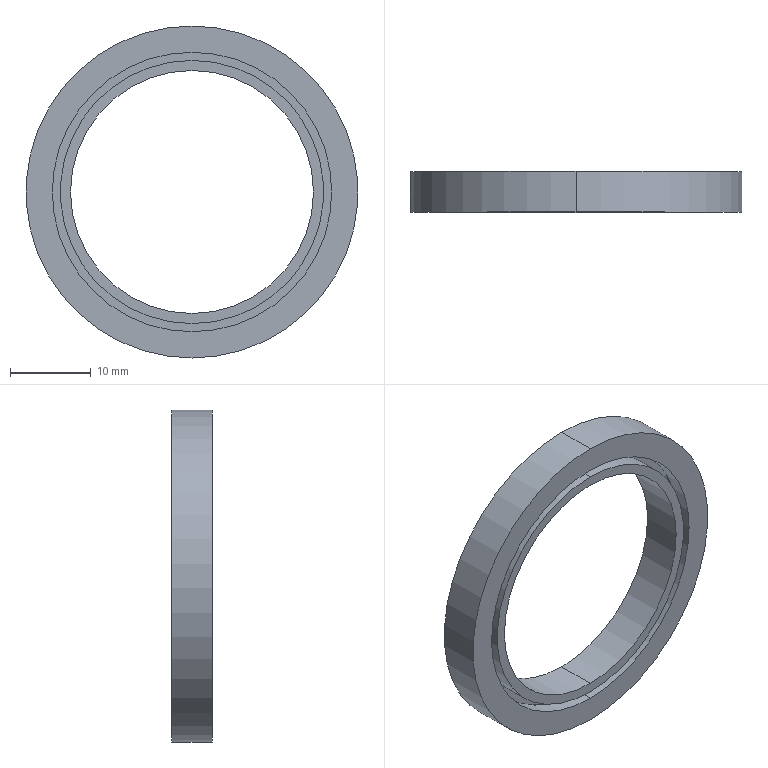Part | SolidWorks | features BossThin 2, Extrusion 1 | 2 solids | 18 faces | box 41 x 5 x 41 mm | volume 2352 mm3 | cylinder 12 | plane 6 | commonest cylinder face diameters 30 x2 32.5 x2 34.5 x2 35.5 x2 37.5 x2 41 x2
STEP:
#1=CARTESIAN_POINT('',(0.,3.,17.75));
#2=VERTEX_POINT('',#1);
#3=CARTESIAN_POINT('',(0.,3.,-17.75));
#4=VERTEX_POINT('',#3);
#5=CARTESIAN_POINT('',(0.,3.,0.));
#6=DIRECTION('',(0.,1.,0.));
#7=DIRECTION('',(1.,0.,0.));
#8=AXIS2_PLACEMENT_3D('',#5,#6,#7);
#9=CIRCLE('',#8,17.75);
#10=EDGE_CURVE('',#2,#4,#9,.T.);
#11=ORIENTED_EDGE('',*,*,#10,.T.);
#12=CARTESIAN_POINT('',(0.,5.,-17.75));
#13=VERTEX_POINT('',#12);
#14=CARTESIAN_POINT('',(0.,3.,-17.75));
#15=DIRECTION('',(0.,1.,0.));
#16=VECTOR('',#15,1000.);
#17=LINE('',#14,#16);
#18=EDGE_CURVE('',#4,#13,#17,.T.);
#19=ORIENTED_EDGE('',*,*,#18,.T.);
#20=CARTESIAN_POINT('',(0.,5.,17.75));
#21=VERTEX_POINT('',#20);
#22=CARTESIAN_POINT('',(0.,5.,0.));
#23=DIRECTION('',(0.,1.,0.));
#24=DIRECTION('',(1.,0.,0.));
#25=AXIS2_PLACEMENT_3D('',#22,#23,#24);
#26=CIRCLE('',#25,17.75);
#27=EDGE_CURVE('',#21,#13,#26,.T.);
#28=ORIENTED_EDGE('',*,*,#27,.F.);
#29=CARTESIAN_POINT('',(0.,3.,17.75));
#30=DIRECTION('',(0.,1.,0.));
#31=VECTOR('',#30,1000.);
#32=LINE('',#29,#31);
#33=EDGE_CURVE('',#2,#21,#32,.T.);
#34=ORIENTED_EDGE('',*,*,#33,.F.);
#35=EDGE_LOOP('',(#11,#19,#28,#34));
#36=FACE_OUTER_BOUND('',#35,.T.);
#37=CARTESIAN_POINT('',(0.,3.,0.));
#38=DIRECTION('',(0.,1.,0.));
#39=DIRECTION('',(0.,0.,1.));
#40=AXIS2_PLACEMENT_3D('',#37,#38,#39);
#41=CYLINDRICAL_SURFACE('',#40,17.75);
#42=ADVANCED_FACE('',(#36),#41,.T.);
#43=CARTESIAN_POINT('',(0.,5.,-15.));
#44=VERTEX_POINT('',#43);
#45=CARTESIAN_POINT('',(0.,5.,15.));
#46=VERTEX_POINT('',#45);
#47=CARTESIAN_POINT('',(0.,5.,0.));
#48=DIRECTION('',(0.,1.,0.));
#49=DIRECTION('',(0.,0.,1.));
#50=AXIS2_PLACEMENT_3D('',#47,#48,#49);
#51=CIRCLE('',#50,15.);
#52=EDGE_CURVE('',#44,#46,#51,.T.);
#53=ORIENTED_EDGE('',*,*,#52,.T.);
#54=CARTESIAN_POINT('',(0.,0.,15.));
#55=VERTEX_POINT('',#54);
#56=CARTESIAN_POINT('',(0.,5.,15.));
#57=DIRECTION('',(0.,-1.,0.));
#58=VECTOR('',#57,1000.);
#59=LINE('',#56,#58);
#60=EDGE_CURVE('',#46,#55,#59,.T.);
#61=ORIENTED_EDGE('',*,*,#60,.T.);
#62=CARTESIAN_POINT('',(0.,0.,-15.));
#63=VERTEX_POINT('',#62);
#64=CARTESIAN_POINT('',(0.,0.,0.));
#65=DIRECTION('',(0.,1.,0.));
#66=DIRECTION('',(0.,0.,1.));
#67=AXIS2_PLACEMENT_3D('',#64,#65,#66);
#68=CIRCLE('',#67,15.);
#69=EDGE_CURVE('',#63,#55,#68,.T.);
#70=ORIENTED_EDGE('',*,*,#69,.F.);
#71=CARTESIAN_POINT('',(0.,5.,-15.));
#72=DIRECTION('',(0.,-1.,0.));
#73=VECTOR('',#72,1000.);
#74=LINE('',#71,#73);
#75=EDGE_CURVE('',#44,#63,#74,.T.);
#76=ORIENTED_EDGE('',*,*,#75,.F.);
#77=EDGE_LOOP('',(#53,#61,#70,#76));
#78=FACE_OUTER_BOUND('',#77,.T.);
#79=CARTESIAN_POINT('',(0.,5.,0.));
#80=DIRECTION('',(0.,-1.,0.));
#81=DIRECTION('',(0.,0.,-1.));
#82=AXIS2_PLACEMENT_3D('',#79,#80,#81);
#83=CYLINDRICAL_SURFACE('',#82,15.);
#84=ADVANCED_FACE('',(#78),#83,.F.);
#85=CARTESIAN_POINT('',(0.,3.,16.25));
#86=VERTEX_POINT('',#85);
#87=CARTESIAN_POINT('',(0.,3.,-16.25));
#88=VERTEX_POINT('',#87);
#89=CARTESIAN_POINT('',(0.,3.,0.));
#90=DIRECTION('',(0.,1.,0.));
#91=DIRECTION('',(0.,0.,1.));
#92=AXIS2_PLACEMENT_3D('',#89,#90,#91);
#93=CIRCLE('',#92,16.25);
#94=EDGE_CURVE('',#86,#88,#93,.T.);
#95=ORIENTED_EDGE('',*,*,#94,.F.);
#96=CARTESIAN_POINT('',(0.,0.,16.25));
#97=VERTEX_POINT('',#96);
#98=CARTESIAN_POINT('',(0.,5.,16.25));
#99=DIRECTION('',(0.,-1.,0.));
#100=VECTOR('',#99,1000.);
#101=LINE('',#98,#100);
#102=EDGE_CURVE('',#86,#97,#101,.T.);
#103=ORIENTED_EDGE('',*,*,#102,.T.);
#104=CARTESIAN_POINT('',(0.,0.,-16.25));
#105=VERTEX_POINT('',#104);
#106=CARTESIAN_POINT('',(0.,0.,0.));
#107=DIRECTION('',(0.,1.,0.));
#108=DIRECTION('',(0.,0.,1.));
#109=AXIS2_PLACEMENT_3D('',#106,#107,#108);
#110=CIRCLE('',#109,16.25);
#111=EDGE_CURVE('',#97,#105,#110,.T.);
#112=ORIENTED_EDGE('',*,*,#111,.T.);
#113=CARTESIAN_POINT('',(0.,5.,-16.25));
#114=DIRECTION('',(0.,-1.,0.));
#115=VECTOR('',#114,1000.);
#116=LINE('',#113,#115);
#117=EDGE_CURVE('',#88,#105,#116,.T.);
#118=ORIENTED_EDGE('',*,*,#117,.F.);
#119=EDGE_LOOP('',(#95,#103,#112,#118));
#120=FACE_OUTER_BOUND('',#119,.T.);
#121=CARTESIAN_POINT('',(0.,5.,0.));
#122=DIRECTION('',(0.,-1.,0.));
#123=DIRECTION('',(0.,0.,-1.));
#124=AXIS2_PLACEMENT_3D('',#121,#122,#123);
#125=CYLINDRICAL_SURFACE('',#124,16.25);
#126=ADVANCED_FACE('',(#120),#125,.T.);
#127=ORIENTED_EDGE('',*,*,#102,.F.);
#128=CARTESIAN_POINT('',(0.,3.,0.));
#129=DIRECTION('',(0.,1.,0.));
#130=DIRECTION('',(0.,0.,1.));
#131=AXIS2_PLACEMENT_3D('',#128,#129,#130);
#132=CIRCLE('',#131,16.25);
#133=EDGE_CURVE('',#88,#86,#132,.T.);
#134=ORIENTED_EDGE('',*,*,#133,.F.);
#135=ORIENTED_EDGE('',*,*,#117,.T.);
#136=CARTESIAN_POINT('',(0.,0.,0.));
#137=DIRECTION('',(0.,1.,0.));
#138=DIRECTION('',(0.,0.,1.));
#139=AXIS2_PLACEMENT_3D('',#136,#137,#138);
#140=CIRCLE('',#139,16.25);
#141=EDGE_CURVE('',#105,#97,#140,.T.);
#142=ORIENTED_EDGE('',*,*,#141,.T.);
#143=EDGE_LOOP('',(#127,#134,#135,#142));
#144=FACE_OUTER_BOUND('',#143,.T.);
#145=CARTESIAN_POINT('',(0.,5.,0.));
#146=DIRECTION('',(0.,-1.,0.));
#147=DIRECTION('',(0.,0.,-1.));
#148=AXIS2_PLACEMENT_3D('',#145,#146,#147);
#149=CYLINDRICAL_SURFACE('',#148,16.25);
#150=ADVANCED_FACE('',(#144),#149,.T.);
#151=ORIENTED_EDGE('',*,*,#60,.F.);
#152=CARTESIAN_POINT('',(0.,5.,0.));
#153=DIRECTION('',(0.,1.,0.));
#154=DIRECTION('',(0.,0.,1.));
#155=AXIS2_PLACEMENT_3D('',#152,#153,#154);
#156=CIRCLE('',#155,15.);
#157=EDGE_CURVE('',#46,#44,#156,.T.);
#158=ORIENTED_EDGE('',*,*,#157,.T.);
#159=ORIENTED_EDGE('',*,*,#75,.T.);
#160=CARTESIAN_POINT('',(0.,0.,0.));
#161=DIRECTION('',(0.,1.,0.));
#162=DIRECTION('',(0.,0.,1.));
#163=AXIS2_PLACEMENT_3D('',#160,#161,#162);
#164=CIRCLE('',#163,15.);
#165=EDGE_CURVE('',#55,#63,#164,.T.);
#166=ORIENTED_EDGE('',*,*,#165,.F.);
#167=EDGE_LOOP('',(#151,#158,#159,#166));
#168=FACE_OUTER_BOUND('',#167,.T.);
#169=CARTESIAN_POINT('',(0.,5.,0.));
#170=DIRECTION('',(0.,-1.,0.));
#171=DIRECTION('',(0.,0.,-1.));
#172=AXIS2_PLACEMENT_3D('',#169,#170,#171);
#173=CYLINDRICAL_SURFACE('',#172,15.);
#174=ADVANCED_FACE('',(#168),#173,.F.);
#175=ORIENTED_EDGE('',*,*,#52,.F.);
#176=ORIENTED_EDGE('',*,*,#157,.F.);
#177=EDGE_LOOP('',(#175,#176));
#178=FACE_BOUND('',#177,.T.);
#179=ORIENTED_EDGE('',*,*,#27,.T.);
#180=CARTESIAN_POINT('',(0.,5.,0.));
#181=DIRECTION('',(0.,1.,0.));
#182=DIRECTION('',(1.,0.,0.));
#183=AXIS2_PLACEMENT_3D('',#180,#181,#182);
#184=CIRCLE('',#183,17.75);
#185=EDGE_CURVE('',#13,#21,#184,.T.);
#186=ORIENTED_EDGE('',*,*,#185,.T.);
#187=EDGE_LOOP('',(#179,#186));
#188=FACE_OUTER_BOUND('',#187,.T.);
#189=CARTESIAN_POINT('',(0.,5.,0.));
#190=DIRECTION('',(0.,1.,0.));
#191=DIRECTION('',(0.,0.,1.));
#192=AXIS2_PLACEMENT_3D('',#189,#190,#191);
#193=PLANE('',#192);
#194=ADVANCED_FACE('',(#178,#188),#193,.T.);
#195=ORIENTED_EDGE('',*,*,#69,.T.);
#196=ORIENTED_EDGE('',*,*,#165,.T.);
#197=EDGE_LOOP('',(#195,#196));
#198=FACE_BOUND('',#197,.T.);
#199=ORIENTED_EDGE('',*,*,#141,.F.);
#200=ORIENTED_EDGE('',*,*,#111,.F.);
#201=EDGE_LOOP('',(#199,#200));
#202=FACE_OUTER_BOUND('',#201,.T.);
#203=CARTESIAN_POINT('',(0.,0.,0.));
#204=DIRECTION('',(0.,1.,0.));
#205=DIRECTION('',(0.,0.,1.));
#206=AXIS2_PLACEMENT_3D('',#203,#204,#205);
#207=PLANE('',#206);
#208=ADVANCED_FACE('',(#198,#202),#207,.F.);
#209=ORIENTED_EDGE('',*,*,#18,.F.);
#210=CARTESIAN_POINT('',(0.,3.,0.));
#211=DIRECTION('',(0.,1.,0.));
#212=DIRECTION('',(1.,0.,0.));
#213=AXIS2_PLACEMENT_3D('',#210,#211,#212);
#214=CIRCLE('',#213,17.75);
#215=EDGE_CURVE('',#4,#2,#214,.T.);
#216=ORIENTED_EDGE('',*,*,#215,.T.);
#217=ORIENTED_EDGE('',*,*,#33,.T.);
#218=ORIENTED_EDGE('',*,*,#185,.F.);
#219=EDGE_LOOP('',(#209,#216,#217,#218));
#220=FACE_OUTER_BOUND('',#219,.T.);
#221=CARTESIAN_POINT('',(0.,3.,0.));
#222=DIRECTION('',(0.,1.,0.));
#223=DIRECTION('',(0.,0.,1.));
#224=AXIS2_PLACEMENT_3D('',#221,#222,#223);
#225=CYLINDRICAL_SURFACE('',#224,17.75);
#226=ADVANCED_FACE('',(#220),#225,.T.);
#227=ORIENTED_EDGE('',*,*,#133,.T.);
#228=ORIENTED_EDGE('',*,*,#94,.T.);
#229=EDGE_LOOP('',(#227,#228));
#230=FACE_BOUND('',#229,.T.);
#231=ORIENTED_EDGE('',*,*,#10,.F.);
#232=ORIENTED_EDGE('',*,*,#215,.F.);
#233=EDGE_LOOP('',(#231,#232));
#234=FACE_OUTER_BOUND('',#233,.T.);
#235=CARTESIAN_POINT('',(0.,3.,0.));
#236=DIRECTION('',(0.,1.,0.));
#237=DIRECTION('',(0.,0.,1.));
#238=AXIS2_PLACEMENT_3D('',#235,#236,#237);
#239=PLANE('',#238);
#240=ADVANCED_FACE('',(#230,#234),#239,.F.);
#241=CLOSED_SHELL('',(#42,#84,#126,#150,#174,#194,#208,#226,#240));
#242=MANIFOLD_SOLID_BREP('',#241);
#243=CARTESIAN_POINT('',(0.,2.,17.25));
#244=VERTEX_POINT('',#243);
#245=CARTESIAN_POINT('',(0.,2.,-17.25));
#246=VERTEX_POINT('',#245);
#247=CARTESIAN_POINT('',(0.,2.,0.));
#248=DIRECTION('',(0.,-1.,0.));
#249=DIRECTION('',(1.,0.,0.));
#250=AXIS2_PLACEMENT_3D('',#247,#248,#249);
#251=CIRCLE('',#250,17.25);
#252=EDGE_CURVE('',#244,#246,#251,.T.);
#253=ORIENTED_EDGE('',*,*,#252,.F.);
#254=CARTESIAN_POINT('',(0.,0.,17.25));
#255=VERTEX_POINT('',#254);
#256=CARTESIAN_POINT('',(0.,2.,17.25));
#257=DIRECTION('',(0.,-1.,0.));
#258=VECTOR('',#257,1000.);
#259=LINE('',#256,#258);
#260=EDGE_CURVE('',#244,#255,#259,.T.);
#261=ORIENTED_EDGE('',*,*,#260,.T.);
#262=CARTESIAN_POINT('',(0.,0.,-17.25));
#263=VERTEX_POINT('',#262);
#264=CARTESIAN_POINT('',(0.,0.,0.));
#265=DIRECTION('',(0.,-1.,0.));
#266=DIRECTION('',(1.,0.,0.));
#267=AXIS2_PLACEMENT_3D('',#264,#265,#266);
#268=CIRCLE('',#267,17.25);
#269=EDGE_CURVE('',#255,#263,#268,.T.);
#270=ORIENTED_EDGE('',*,*,#269,.T.);
#271=CARTESIAN_POINT('',(0.,2.,-17.25));
#272=DIRECTION('',(0.,-1.,0.));
#273=VECTOR('',#272,1000.);
#274=LINE('',#271,#273);
#275=EDGE_CURVE('',#246,#263,#274,.T.);
#276=ORIENTED_EDGE('',*,*,#275,.F.);
#277=EDGE_LOOP('',(#253,#261,#270,#276));
#278=FACE_OUTER_BOUND('',#277,.T.);
#279=CARTESIAN_POINT('',(0.,2.,0.));
#280=DIRECTION('',(0.,-1.,0.));
#281=DIRECTION('',(0.,0.,-1.));
#282=AXIS2_PLACEMENT_3D('',#279,#280,#281);
#283=CYLINDRICAL_SURFACE('',#282,17.25);
#284=ADVANCED_FACE('',(#278),#283,.F.);
#285=CARTESIAN_POINT('',(0.,5.,20.5));
#286=VERTEX_POINT('',#285);
#287=CARTESIAN_POINT('',(0.,5.,-20.5));
#288=VERTEX_POINT('',#287);
#289=CARTESIAN_POINT('',(0.,5.,0.));
#290=DIRECTION('',(0.,1.,0.));
#291=DIRECTION('',(0.,0.,1.));
#292=AXIS2_PLACEMENT_3D('',#289,#290,#291);
#293=CIRCLE('',#292,20.5);
#294=EDGE_CURVE('',#286,#288,#293,.T.);
#295=ORIENTED_EDGE('',*,*,#294,.F.);
#296=CARTESIAN_POINT('',(0.,0.,20.5));
#297=VERTEX_POINT('',#296);
#298=CARTESIAN_POINT('',(0.,5.,20.5));
#299=DIRECTION('',(0.,-1.,0.));
#300=VECTOR('',#299,1000.);
#301=LINE('',#298,#300);
#302=EDGE_CURVE('',#286,#297,#301,.T.);
#303=ORIENTED_EDGE('',*,*,#302,.T.);
#304=CARTESIAN_POINT('',(0.,0.,-20.5));
#305=VERTEX_POINT('',#304);
#306=CARTESIAN_POINT('',(0.,0.,0.));
#307=DIRECTION('',(0.,1.,0.));
#308=DIRECTION('',(0.,0.,1.));
#309=AXIS2_PLACEMENT_3D('',#306,#307,#308);
#310=CIRCLE('',#309,20.5);
#311=EDGE_CURVE('',#297,#305,#310,.T.);
#312=ORIENTED_EDGE('',*,*,#311,.T.);
#313=CARTESIAN_POINT('',(0.,5.,-20.5));
#314=DIRECTION('',(0.,-1.,0.));
#315=VECTOR('',#314,1000.);
#316=LINE('',#313,#315);
#317=EDGE_CURVE('',#288,#305,#316,.T.);
#318=ORIENTED_EDGE('',*,*,#317,.F.);
#319=EDGE_LOOP('',(#295,#303,#312,#318));
#320=FACE_OUTER_BOUND('',#319,.T.);
#321=CARTESIAN_POINT('',(0.,5.,0.));
#322=DIRECTION('',(0.,-1.,0.));
#323=DIRECTION('',(0.,0.,-1.));
#324=AXIS2_PLACEMENT_3D('',#321,#322,#323);
#325=CYLINDRICAL_SURFACE('',#324,20.5);
#326=ADVANCED_FACE('',(#320),#325,.T.);
#327=CARTESIAN_POINT('',(0.,5.,-18.75));
#328=VERTEX_POINT('',#327);
#329=CARTESIAN_POINT('',(0.,5.,18.75));
#330=VERTEX_POINT('',#329);
#331=CARTESIAN_POINT('',(0.,5.,0.));
#332=DIRECTION('',(0.,1.,0.));
#333=DIRECTION('',(0.,0.,1.));
#334=AXIS2_PLACEMENT_3D('',#331,#332,#333);
#335=CIRCLE('',#334,18.75);
#336=EDGE_CURVE('',#328,#330,#335,.T.);
#337=ORIENTED_EDGE('',*,*,#336,.T.);
#338=CARTESIAN_POINT('',(0.,2.,18.75));
#339=VERTEX_POINT('',#338);
#340=CARTESIAN_POINT('',(0.,5.,18.75));
#341=DIRECTION('',(0.,-1.,0.));
#342=VECTOR('',#341,1000.);
#343=LINE('',#340,#342);
#344=EDGE_CURVE('',#330,#339,#343,.T.);
#345=ORIENTED_EDGE('',*,*,#344,.T.);
#346=CARTESIAN_POINT('',(0.,2.,-18.75));
#347=VERTEX_POINT('',#346);
#348=CARTESIAN_POINT('',(0.,2.,0.));
#349=DIRECTION('',(0.,-1.,0.));
#350=DIRECTION('',(0.,0.,-1.));
#351=AXIS2_PLACEMENT_3D('',#348,#349,#350);
#352=CIRCLE('',#351,18.75);
#353=EDGE_CURVE('',#339,#347,#352,.T.);
#354=ORIENTED_EDGE('',*,*,#353,.T.);
#355=CARTESIAN_POINT('',(0.,5.,-18.75));
#356=DIRECTION('',(0.,-1.,0.));
#357=VECTOR('',#356,1000.);
#358=LINE('',#355,#357);
#359=EDGE_CURVE('',#328,#347,#358,.T.);
#360=ORIENTED_EDGE('',*,*,#359,.F.);
#361=EDGE_LOOP('',(#337,#345,#354,#360));
#362=FACE_OUTER_BOUND('',#361,.T.);
#363=CARTESIAN_POINT('',(0.,5.,0.));
#364=DIRECTION('',(0.,-1.,0.));
#365=DIRECTION('',(0.,0.,-1.));
#366=AXIS2_PLACEMENT_3D('',#363,#364,#365);
#367=CYLINDRICAL_SURFACE('',#366,18.75);
#368=ADVANCED_FACE('',(#362),#367,.F.);
#369=ORIENTED_EDGE('',*,*,#344,.F.);
#370=CARTESIAN_POINT('',(0.,5.,0.));
#371=DIRECTION('',(0.,1.,0.));
#372=DIRECTION('',(0.,0.,1.));
#373=AXIS2_PLACEMENT_3D('',#370,#371,#372);
#374=CIRCLE('',#373,18.75);
#375=EDGE_CURVE('',#330,#328,#374,.T.);
#376=ORIENTED_EDGE('',*,*,#375,.T.);
#377=ORIENTED_EDGE('',*,*,#359,.T.);
#378=CARTESIAN_POINT('',(0.,2.,0.));
#379=DIRECTION('',(0.,-1.,0.));
#380=DIRECTION('',(0.,0.,-1.));
#381=AXIS2_PLACEMENT_3D('',#378,#379,#380);
#382=CIRCLE('',#381,18.75);
#383=EDGE_CURVE('',#347,#339,#382,.T.);
#384=ORIENTED_EDGE('',*,*,#383,.T.);
#385=EDGE_LOOP('',(#369,#376,#377,#384));
#386=FACE_OUTER_BOUND('',#385,.T.);
#387=CARTESIAN_POINT('',(0.,5.,0.));
#388=DIRECTION('',(0.,-1.,0.));
#389=DIRECTION('',(0.,0.,-1.));
#390=AXIS2_PLACEMENT_3D('',#387,#388,#389);
#391=CYLINDRICAL_SURFACE('',#390,18.75);
#392=ADVANCED_FACE('',(#386),#391,.F.);
#393=ORIENTED_EDGE('',*,*,#302,.F.);
#394=CARTESIAN_POINT('',(0.,5.,0.));
#395=DIRECTION('',(0.,1.,0.));
#396=DIRECTION('',(0.,0.,1.));
#397=AXIS2_PLACEMENT_3D('',#394,#395,#396);
#398=CIRCLE('',#397,20.5);
#399=EDGE_CURVE('',#288,#286,#398,.T.);
#400=ORIENTED_EDGE('',*,*,#399,.F.);
#401=ORIENTED_EDGE('',*,*,#317,.T.);
#402=CARTESIAN_POINT('',(0.,0.,0.));
#403=DIRECTION('',(0.,1.,0.));
#404=DIRECTION('',(0.,0.,1.));
#405=AXIS2_PLACEMENT_3D('',#402,#403,#404);
#406=CIRCLE('',#405,20.5);
#407=EDGE_CURVE('',#305,#297,#406,.T.);
#408=ORIENTED_EDGE('',*,*,#407,.T.);
#409=EDGE_LOOP('',(#393,#400,#401,#408));
#410=FACE_OUTER_BOUND('',#409,.T.);
#411=CARTESIAN_POINT('',(0.,5.,0.));
#412=DIRECTION('',(0.,-1.,0.));
#413=DIRECTION('',(0.,0.,-1.));
#414=AXIS2_PLACEMENT_3D('',#411,#412,#413);
#415=CYLINDRICAL_SURFACE('',#414,20.5);
#416=ADVANCED_FACE('',(#410),#415,.T.);
#417=ORIENTED_EDGE('',*,*,#336,.F.);
#418=ORIENTED_EDGE('',*,*,#375,.F.);
#419=EDGE_LOOP('',(#417,#418));
#420=FACE_BOUND('',#419,.T.);
#421=ORIENTED_EDGE('',*,*,#399,.T.);
#422=ORIENTED_EDGE('',*,*,#294,.T.);
#423=EDGE_LOOP('',(#421,#422));
#424=FACE_OUTER_BOUND('',#423,.T.);
#425=CARTESIAN_POINT('',(0.,5.,0.));
#426=DIRECTION('',(0.,1.,0.));
#427=DIRECTION('',(0.,0.,1.));
#428=AXIS2_PLACEMENT_3D('',#425,#426,#427);
#429=PLANE('',#428);
#430=ADVANCED_FACE('',(#420,#424),#429,.T.);
#431=ORIENTED_EDGE('',*,*,#407,.F.);
#432=ORIENTED_EDGE('',*,*,#311,.F.);
#433=EDGE_LOOP('',(#431,#432));
#434=FACE_OUTER_BOUND('',#433,.T.);
#435=CARTESIAN_POINT('',(0.,0.,0.));
#436=DIRECTION('',(0.,-1.,0.));
#437=DIRECTION('',(1.,0.,0.));
#438=AXIS2_PLACEMENT_3D('',#435,#436,#437);
#439=CIRCLE('',#438,17.25);
#440=EDGE_CURVE('',#263,#255,#439,.T.);
#441=ORIENTED_EDGE('',*,*,#440,.F.);
#442=ORIENTED_EDGE('',*,*,#269,.F.);
#443=EDGE_LOOP('',(#441,#442));
#444=FACE_BOUND('',#443,.T.);
#445=CARTESIAN_POINT('',(0.,0.,0.));
#446=DIRECTION('',(0.,1.,0.));
#447=DIRECTION('',(0.,0.,1.));
#448=AXIS2_PLACEMENT_3D('',#445,#446,#447);
#449=PLANE('',#448);
#450=ADVANCED_FACE('',(#434,#444),#449,.F.);
#451=CARTESIAN_POINT('',(0.,2.,0.));
#452=DIRECTION('',(0.,-1.,0.));
#453=DIRECTION('',(1.,0.,0.));
#454=AXIS2_PLACEMENT_3D('',#451,#452,#453);
#455=CIRCLE('',#454,17.25);
#456=EDGE_CURVE('',#246,#244,#455,.T.);
#457=ORIENTED_EDGE('',*,*,#456,.T.);
#458=ORIENTED_EDGE('',*,*,#252,.T.);
#459=EDGE_LOOP('',(#457,#458));
#460=FACE_BOUND('',#459,.T.);
#461=ORIENTED_EDGE('',*,*,#383,.F.);
#462=ORIENTED_EDGE('',*,*,#353,.F.);
#463=EDGE_LOOP('',(#461,#462));
#464=FACE_OUTER_BOUND('',#463,.T.);
#465=CARTESIAN_POINT('',(0.,2.,0.));
#466=DIRECTION('',(0.,-1.,0.));
#467=DIRECTION('',(0.,0.,-1.));
#468=AXIS2_PLACEMENT_3D('',#465,#466,#467);
#469=PLANE('',#468);
#470=ADVANCED_FACE('',(#460,#464),#469,.F.);
#471=ORIENTED_EDGE('',*,*,#260,.F.);
#472=ORIENTED_EDGE('',*,*,#456,.F.);
#473=ORIENTED_EDGE('',*,*,#275,.T.);
#474=ORIENTED_EDGE('',*,*,#440,.T.);
#475=EDGE_LOOP('',(#471,#472,#473,#474));
#476=FACE_OUTER_BOUND('',#475,.T.);
#477=CARTESIAN_POINT('',(0.,2.,0.));
#478=DIRECTION('',(0.,-1.,0.));
#479=DIRECTION('',(0.,0.,-1.));
#480=AXIS2_PLACEMENT_3D('',#477,#478,#479);
#481=CYLINDRICAL_SURFACE('',#480,17.25);
#482=ADVANCED_FACE('',(#476),#481,.F.);
#483=CLOSED_SHELL('',(#284,#326,#368,#392,#416,#430,#450,#470,#482));
#484=MANIFOLD_SOLID_BREP('',#483);
#485=CARTESIAN_POINT('',(0.,0.,0.));
#486=DIRECTION('',(0.,0.,1.));
#487=DIRECTION('',(1.,0.,0.));
#488=AXIS2_PLACEMENT_3D('',#485,#486,#487);
#489=(LENGTH_UNIT()NAMED_UNIT(*)SI_UNIT(.MILLI.,.METRE.));
#490=UNCERTAINTY_MEASURE_WITH_UNIT(LENGTH_MEASURE(0.00001),#489,'','');
#491=(NAMED_UNIT(*)PLANE_ANGLE_UNIT()SI_UNIT($,.RADIAN.));
#492=(NAMED_UNIT(*)SI_UNIT($,.STERADIAN.)SOLID_ANGLE_UNIT());
#493=(GEOMETRIC_REPRESENTATION_CONTEXT(3)GLOBAL_UNCERTAINTY_ASSIGNED_CONTEXT((#490))GLOBAL_UNIT_ASSIGNED_CONTEXT((#489,#491,#492))REPRESENTATION_CONTEXT('',''));
#494=ADVANCED_BREP_SHAPE_REPRESENTATION('',(#242,#484,#488),#493);